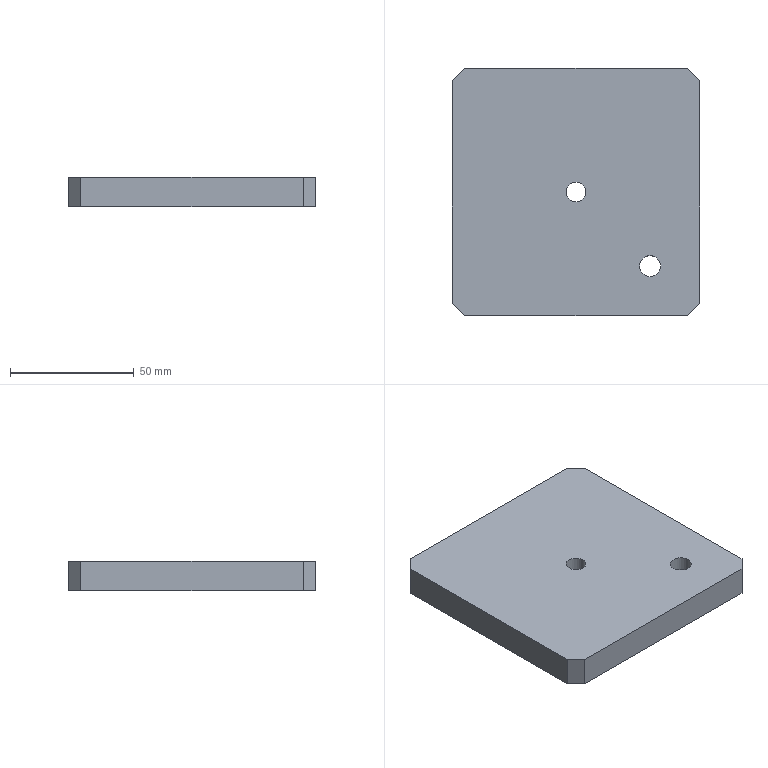Part | NX | features BREP 1 | 1 solid | 12 faces | box 100 x 100 x 12 mm | volume 118116 mm3 | plane 10 | cylinder 2 | commonest cylinder face diameters 8 x1 8.5 x1
STEP:
#1=CARTESIAN_POINT('',(50.,-45.,12.));
#2=VERTEX_POINT('',#1);
#3=CARTESIAN_POINT('',(50.,45.,12.));
#4=VERTEX_POINT('',#3);
#5=CARTESIAN_POINT('',(50.,-100.,12.));
#6=DIRECTION('',(0.,1.,0.));
#7=VECTOR('',#6,1000.);
#8=LINE('',#5,#7);
#9=EDGE_CURVE('',#2,#4,#8,.T.);
#10=ORIENTED_EDGE('',*,*,#9,.F.);
#11=CARTESIAN_POINT('',(50.,-45.,0.));
#12=VERTEX_POINT('',#11);
#13=CARTESIAN_POINT('',(50.,-45.,15.));
#14=DIRECTION('',(0.,0.,-1.));
#15=VECTOR('',#14,1000.);
#16=LINE('',#13,#15);
#17=EDGE_CURVE('',#2,#12,#16,.T.);
#18=ORIENTED_EDGE('',*,*,#17,.T.);
#19=CARTESIAN_POINT('',(50.,45.,0.));
#20=VERTEX_POINT('',#19);
#21=CARTESIAN_POINT('',(50.,50.,0.));
#22=DIRECTION('',(0.,1.,0.));
#23=VECTOR('',#22,1000.);
#24=LINE('',#21,#23);
#25=EDGE_CURVE('',#12,#20,#24,.T.);
#26=ORIENTED_EDGE('',*,*,#25,.T.);
#27=CARTESIAN_POINT('',(50.,45.,15.));
#28=DIRECTION('',(0.,0.,1.));
#29=VECTOR('',#28,1000.);
#30=LINE('',#27,#29);
#31=EDGE_CURVE('',#20,#4,#30,.T.);
#32=ORIENTED_EDGE('',*,*,#31,.T.);
#33=EDGE_LOOP('',(#10,#18,#26,#32));
#34=FACE_BOUND('',#33,.T.);
#35=CARTESIAN_POINT('',(50.,50.,15.));
#36=DIRECTION('',(-1.,0.,0.));
#37=DIRECTION('',(0.,0.,-1.));
#38=AXIS2_PLACEMENT_3D('',#35,#36,#37);
#39=PLANE('',#38);
#40=ADVANCED_FACE('',(#34),#39,.F.);
#41=CARTESIAN_POINT('',(45.,50.,12.));
#42=VERTEX_POINT('',#41);
#43=CARTESIAN_POINT('',(-45.,50.,12.));
#44=VERTEX_POINT('',#43);
#45=CARTESIAN_POINT('',(-50.,50.,12.));
#46=DIRECTION('',(-1.,0.,0.));
#47=VECTOR('',#46,1000.);
#48=LINE('',#45,#47);
#49=EDGE_CURVE('',#42,#44,#48,.T.);
#50=ORIENTED_EDGE('',*,*,#49,.F.);
#51=CARTESIAN_POINT('',(45.,50.,0.));
#52=VERTEX_POINT('',#51);
#53=CARTESIAN_POINT('',(45.,50.,15.));
#54=DIRECTION('',(0.,0.,-1.));
#55=VECTOR('',#54,1000.);
#56=LINE('',#53,#55);
#57=EDGE_CURVE('',#42,#52,#56,.T.);
#58=ORIENTED_EDGE('',*,*,#57,.T.);
#59=CARTESIAN_POINT('',(-45.,50.,0.));
#60=VERTEX_POINT('',#59);
#61=CARTESIAN_POINT('',(-50.,50.,0.));
#62=DIRECTION('',(-1.,0.,0.));
#63=VECTOR('',#62,1000.);
#64=LINE('',#61,#63);
#65=EDGE_CURVE('',#52,#60,#64,.T.);
#66=ORIENTED_EDGE('',*,*,#65,.T.);
#67=CARTESIAN_POINT('',(-45.,50.,15.));
#68=DIRECTION('',(0.,0.,1.));
#69=VECTOR('',#68,1000.);
#70=LINE('',#67,#69);
#71=EDGE_CURVE('',#60,#44,#70,.T.);
#72=ORIENTED_EDGE('',*,*,#71,.T.);
#73=EDGE_LOOP('',(#50,#58,#66,#72));
#74=FACE_BOUND('',#73,.T.);
#75=CARTESIAN_POINT('',(-50.,50.,15.));
#76=DIRECTION('',(0.,-1.,0.));
#77=DIRECTION('',(0.,0.,1.));
#78=AXIS2_PLACEMENT_3D('',#75,#76,#77);
#79=PLANE('',#78);
#80=ADVANCED_FACE('',(#74),#79,.F.);
#81=CARTESIAN_POINT('',(-50.,45.,12.));
#82=VERTEX_POINT('',#81);
#83=CARTESIAN_POINT('',(-50.,-45.,12.));
#84=VERTEX_POINT('',#83);
#85=CARTESIAN_POINT('',(-50.,50.,12.));
#86=DIRECTION('',(0.,-1.,0.));
#87=VECTOR('',#86,1000.);
#88=LINE('',#85,#87);
#89=EDGE_CURVE('',#82,#84,#88,.T.);
#90=ORIENTED_EDGE('',*,*,#89,.F.);
#91=CARTESIAN_POINT('',(-50.,45.,0.));
#92=VERTEX_POINT('',#91);
#93=CARTESIAN_POINT('',(-50.,45.,15.));
#94=DIRECTION('',(0.,0.,-1.));
#95=VECTOR('',#94,1000.);
#96=LINE('',#93,#95);
#97=EDGE_CURVE('',#82,#92,#96,.T.);
#98=ORIENTED_EDGE('',*,*,#97,.T.);
#99=CARTESIAN_POINT('',(-50.,-45.,0.));
#100=VERTEX_POINT('',#99);
#101=CARTESIAN_POINT('',(-50.,50.,0.));
#102=DIRECTION('',(0.,-1.,0.));
#103=VECTOR('',#102,1000.);
#104=LINE('',#101,#103);
#105=EDGE_CURVE('',#92,#100,#104,.T.);
#106=ORIENTED_EDGE('',*,*,#105,.T.);
#107=CARTESIAN_POINT('',(-50.,-45.,15.));
#108=DIRECTION('',(0.,0.,1.));
#109=VECTOR('',#108,1000.);
#110=LINE('',#107,#109);
#111=EDGE_CURVE('',#100,#84,#110,.T.);
#112=ORIENTED_EDGE('',*,*,#111,.T.);
#113=EDGE_LOOP('',(#90,#98,#106,#112));
#114=FACE_BOUND('',#113,.T.);
#115=CARTESIAN_POINT('',(-50.,50.,15.));
#116=DIRECTION('',(1.,0.,0.));
#117=DIRECTION('',(0.,-1.,0.));
#118=AXIS2_PLACEMENT_3D('',#115,#116,#117);
#119=PLANE('',#118);
#120=ADVANCED_FACE('',(#114),#119,.F.);
#121=CARTESIAN_POINT('',(-45.,-50.,12.));
#122=VERTEX_POINT('',#121);
#123=CARTESIAN_POINT('',(45.,-50.,12.));
#124=VERTEX_POINT('',#123);
#125=CARTESIAN_POINT('',(-50.,-50.,12.));
#126=DIRECTION('',(1.,0.,0.));
#127=VECTOR('',#126,1000.);
#128=LINE('',#125,#127);
#129=EDGE_CURVE('',#122,#124,#128,.T.);
#130=ORIENTED_EDGE('',*,*,#129,.F.);
#131=CARTESIAN_POINT('',(-45.,-50.,0.));
#132=VERTEX_POINT('',#131);
#133=CARTESIAN_POINT('',(-45.,-50.,15.));
#134=DIRECTION('',(0.,0.,-1.));
#135=VECTOR('',#134,1000.);
#136=LINE('',#133,#135);
#137=EDGE_CURVE('',#122,#132,#136,.T.);
#138=ORIENTED_EDGE('',*,*,#137,.T.);
#139=CARTESIAN_POINT('',(45.,-50.,0.));
#140=VERTEX_POINT('',#139);
#141=CARTESIAN_POINT('',(-50.,-50.,0.));
#142=DIRECTION('',(1.,0.,0.));
#143=VECTOR('',#142,1000.);
#144=LINE('',#141,#143);
#145=EDGE_CURVE('',#132,#140,#144,.T.);
#146=ORIENTED_EDGE('',*,*,#145,.T.);
#147=CARTESIAN_POINT('',(45.,-50.,15.));
#148=DIRECTION('',(0.,0.,1.));
#149=VECTOR('',#148,1000.);
#150=LINE('',#147,#149);
#151=EDGE_CURVE('',#140,#124,#150,.T.);
#152=ORIENTED_EDGE('',*,*,#151,.T.);
#153=EDGE_LOOP('',(#130,#138,#146,#152));
#154=FACE_BOUND('',#153,.T.);
#155=CARTESIAN_POINT('',(-50.,-50.,15.));
#156=DIRECTION('',(0.,1.,0.));
#157=DIRECTION('',(0.,0.,-1.));
#158=AXIS2_PLACEMENT_3D('',#155,#156,#157);
#159=PLANE('',#158);
#160=ADVANCED_FACE('',(#154),#159,.F.);
#161=ORIENTED_EDGE('',*,*,#137,.F.);
#162=CARTESIAN_POINT('',(-45.,-50.,12.));
#163=DIRECTION('',(-0.7071,0.7071,0.));
#164=VECTOR('',#163,1000.);
#165=LINE('',#162,#164);
#166=EDGE_CURVE('',#122,#84,#165,.T.);
#167=ORIENTED_EDGE('',*,*,#166,.T.);
#168=ORIENTED_EDGE('',*,*,#111,.F.);
#169=CARTESIAN_POINT('',(-45.,-50.,0.));
#170=DIRECTION('',(-0.7071,0.7071,0.));
#171=VECTOR('',#170,1000.);
#172=LINE('',#169,#171);
#173=EDGE_CURVE('',#132,#100,#172,.T.);
#174=ORIENTED_EDGE('',*,*,#173,.F.);
#175=EDGE_LOOP('',(#161,#167,#168,#174));
#176=FACE_BOUND('',#175,.T.);
#177=CARTESIAN_POINT('',(-45.,-50.,15.));
#178=DIRECTION('',(0.7071,0.7071,0.));
#179=DIRECTION('',(0.,0.,1.));
#180=AXIS2_PLACEMENT_3D('',#177,#178,#179);
#181=PLANE('',#180);
#182=ADVANCED_FACE('',(#176),#181,.F.);
#183=ORIENTED_EDGE('',*,*,#17,.F.);
#184=CARTESIAN_POINT('',(50.,-45.,12.));
#185=DIRECTION('',(-0.7071,-0.7071,0.));
#186=VECTOR('',#185,1000.);
#187=LINE('',#184,#186);
#188=EDGE_CURVE('',#2,#124,#187,.T.);
#189=ORIENTED_EDGE('',*,*,#188,.T.);
#190=ORIENTED_EDGE('',*,*,#151,.F.);
#191=CARTESIAN_POINT('',(50.,-45.,0.));
#192=DIRECTION('',(-0.7071,-0.7071,0.));
#193=VECTOR('',#192,1000.);
#194=LINE('',#191,#193);
#195=EDGE_CURVE('',#12,#140,#194,.T.);
#196=ORIENTED_EDGE('',*,*,#195,.F.);
#197=EDGE_LOOP('',(#183,#189,#190,#196));
#198=FACE_BOUND('',#197,.T.);
#199=CARTESIAN_POINT('',(50.,-45.,15.));
#200=DIRECTION('',(-0.7071,0.7071,0.));
#201=DIRECTION('',(0.,0.,1.));
#202=AXIS2_PLACEMENT_3D('',#199,#200,#201);
#203=PLANE('',#202);
#204=ADVANCED_FACE('',(#198),#203,.F.);
#205=ORIENTED_EDGE('',*,*,#57,.F.);
#206=CARTESIAN_POINT('',(45.,50.,12.));
#207=DIRECTION('',(0.7071,-0.7071,0.));
#208=VECTOR('',#207,1000.);
#209=LINE('',#206,#208);
#210=EDGE_CURVE('',#42,#4,#209,.T.);
#211=ORIENTED_EDGE('',*,*,#210,.T.);
#212=ORIENTED_EDGE('',*,*,#31,.F.);
#213=CARTESIAN_POINT('',(45.,50.,0.));
#214=DIRECTION('',(0.7071,-0.7071,0.));
#215=VECTOR('',#214,1000.);
#216=LINE('',#213,#215);
#217=EDGE_CURVE('',#52,#20,#216,.T.);
#218=ORIENTED_EDGE('',*,*,#217,.F.);
#219=EDGE_LOOP('',(#205,#211,#212,#218));
#220=FACE_BOUND('',#219,.T.);
#221=CARTESIAN_POINT('',(45.,50.,15.));
#222=DIRECTION('',(-0.7071,-0.7071,0.));
#223=DIRECTION('',(0.,0.,1.));
#224=AXIS2_PLACEMENT_3D('',#221,#222,#223);
#225=PLANE('',#224);
#226=ADVANCED_FACE('',(#220),#225,.F.);
#227=ORIENTED_EDGE('',*,*,#97,.F.);
#228=CARTESIAN_POINT('',(-50.,45.,12.));
#229=DIRECTION('',(0.7071,0.7071,0.));
#230=VECTOR('',#229,1000.);
#231=LINE('',#228,#230);
#232=EDGE_CURVE('',#82,#44,#231,.T.);
#233=ORIENTED_EDGE('',*,*,#232,.T.);
#234=ORIENTED_EDGE('',*,*,#71,.F.);
#235=CARTESIAN_POINT('',(-50.,45.,0.));
#236=DIRECTION('',(0.7071,0.7071,0.));
#237=VECTOR('',#236,1000.);
#238=LINE('',#235,#237);
#239=EDGE_CURVE('',#92,#60,#238,.T.);
#240=ORIENTED_EDGE('',*,*,#239,.F.);
#241=EDGE_LOOP('',(#227,#233,#234,#240));
#242=FACE_BOUND('',#241,.T.);
#243=CARTESIAN_POINT('',(-50.,45.,15.));
#244=DIRECTION('',(0.7071,-0.7071,0.));
#245=DIRECTION('',(0.,0.,1.));
#246=AXIS2_PLACEMENT_3D('',#243,#244,#245);
#247=PLANE('',#246);
#248=ADVANCED_FACE('',(#242),#247,.F.);
#249=CARTESIAN_POINT('',(34.25,-30.,0.));
#250=VERTEX_POINT('',#249);
#251=CARTESIAN_POINT('',(30.,-30.,0.));
#252=DIRECTION('',(0.,0.,1.));
#253=DIRECTION('',(1.,0.,0.));
#254=AXIS2_PLACEMENT_3D('',#251,#252,#253);
#255=CIRCLE('',#254,4.25);
#256=EDGE_CURVE('',#250,#250,#255,.T.);
#257=ORIENTED_EDGE('',*,*,#256,.T.);
#258=EDGE_LOOP('',(#257));
#259=FACE_BOUND('',#258,.T.);
#260=CARTESIAN_POINT('',(4.,0.,0.));
#261=VERTEX_POINT('',#260);
#262=CARTESIAN_POINT('',(0.,0.,0.));
#263=DIRECTION('',(0.,0.,1.));
#264=DIRECTION('',(1.,0.,0.));
#265=AXIS2_PLACEMENT_3D('',#262,#263,#264);
#266=CIRCLE('',#265,4.);
#267=EDGE_CURVE('',#261,#261,#266,.T.);
#268=ORIENTED_EDGE('',*,*,#267,.T.);
#269=EDGE_LOOP('',(#268));
#270=FACE_BOUND('',#269,.T.);
#271=ORIENTED_EDGE('',*,*,#145,.F.);
#272=ORIENTED_EDGE('',*,*,#173,.T.);
#273=ORIENTED_EDGE('',*,*,#105,.F.);
#274=ORIENTED_EDGE('',*,*,#239,.T.);
#275=ORIENTED_EDGE('',*,*,#65,.F.);
#276=ORIENTED_EDGE('',*,*,#217,.T.);
#277=ORIENTED_EDGE('',*,*,#25,.F.);
#278=ORIENTED_EDGE('',*,*,#195,.T.);
#279=EDGE_LOOP('',(#271,#272,#273,#274,#275,#276,#277,#278));
#280=FACE_BOUND('',#279,.T.);
#281=CARTESIAN_POINT('',(0.,0.,0.));
#282=DIRECTION('',(0.,0.,1.));
#283=DIRECTION('',(-1.,0.,0.));
#284=AXIS2_PLACEMENT_3D('',#281,#282,#283);
#285=PLANE('',#284);
#286=ADVANCED_FACE('',(#259,#270,#280),#285,.F.);
#287=CARTESIAN_POINT('',(34.25,-30.,12.));
#288=VERTEX_POINT('',#287);
#289=CARTESIAN_POINT('',(30.,-30.,12.));
#290=DIRECTION('',(0.,0.,1.));
#291=DIRECTION('',(1.,0.,0.));
#292=AXIS2_PLACEMENT_3D('',#289,#290,#291);
#293=CIRCLE('',#292,4.25);
#294=EDGE_CURVE('',#288,#288,#293,.T.);
#295=ORIENTED_EDGE('',*,*,#294,.F.);
#296=EDGE_LOOP('',(#295));
#297=FACE_BOUND('',#296,.T.);
#298=CARTESIAN_POINT('',(4.,0.,12.));
#299=VERTEX_POINT('',#298);
#300=CARTESIAN_POINT('',(0.,0.,12.));
#301=DIRECTION('',(0.,0.,1.));
#302=DIRECTION('',(1.,0.,0.));
#303=AXIS2_PLACEMENT_3D('',#300,#301,#302);
#304=CIRCLE('',#303,4.);
#305=EDGE_CURVE('',#299,#299,#304,.T.);
#306=ORIENTED_EDGE('',*,*,#305,.F.);
#307=EDGE_LOOP('',(#306));
#308=FACE_BOUND('',#307,.T.);
#309=ORIENTED_EDGE('',*,*,#9,.T.);
#310=ORIENTED_EDGE('',*,*,#210,.F.);
#311=ORIENTED_EDGE('',*,*,#49,.T.);
#312=ORIENTED_EDGE('',*,*,#232,.F.);
#313=ORIENTED_EDGE('',*,*,#89,.T.);
#314=ORIENTED_EDGE('',*,*,#166,.F.);
#315=ORIENTED_EDGE('',*,*,#129,.T.);
#316=ORIENTED_EDGE('',*,*,#188,.F.);
#317=EDGE_LOOP('',(#309,#310,#311,#312,#313,#314,#315,#316));
#318=FACE_BOUND('',#317,.T.);
#319=CARTESIAN_POINT('',(-900.,250.,12.));
#320=DIRECTION('',(0.,0.,1.));
#321=DIRECTION('',(-1.,0.,0.));
#322=AXIS2_PLACEMENT_3D('',#319,#320,#321);
#323=PLANE('',#322);
#324=ADVANCED_FACE('',(#297,#308,#318),#323,.T.);
#325=ORIENTED_EDGE('',*,*,#305,.T.);
#326=EDGE_LOOP('',(#325));
#327=FACE_BOUND('',#326,.T.);
#328=ORIENTED_EDGE('',*,*,#267,.F.);
#329=EDGE_LOOP('',(#328));
#330=FACE_BOUND('',#329,.T.);
#331=CARTESIAN_POINT('',(0.,0.,12.));
#332=DIRECTION('',(0.,0.,1.));
#333=DIRECTION('',(-1.,0.,0.));
#334=AXIS2_PLACEMENT_3D('',#331,#332,#333);
#335=CYLINDRICAL_SURFACE('',#334,4.);
#336=ADVANCED_FACE('',(#327,#330),#335,.F.);
#337=ORIENTED_EDGE('',*,*,#294,.T.);
#338=EDGE_LOOP('',(#337));
#339=FACE_BOUND('',#338,.T.);
#340=ORIENTED_EDGE('',*,*,#256,.F.);
#341=EDGE_LOOP('',(#340));
#342=FACE_BOUND('',#341,.T.);
#343=CARTESIAN_POINT('',(30.,-30.,12.));
#344=DIRECTION('',(0.,0.,1.));
#345=DIRECTION('',(-1.,0.,0.));
#346=AXIS2_PLACEMENT_3D('',#343,#344,#345);
#347=CYLINDRICAL_SURFACE('',#346,4.25);
#348=ADVANCED_FACE('',(#339,#342),#347,.F.);
#349=CLOSED_SHELL('',(#40,#80,#120,#160,#182,#204,#226,#248,#286,#324,#336,#348));
#350=MANIFOLD_SOLID_BREP('',#349);
#351=(LENGTH_UNIT()NAMED_UNIT(*)SI_UNIT(.MILLI.,.METRE.));
#352=UNCERTAINTY_MEASURE_WITH_UNIT(LENGTH_MEASURE(0.00001),#351,'','');
#353=(NAMED_UNIT(*)PLANE_ANGLE_UNIT()SI_UNIT($,.RADIAN.));
#354=(NAMED_UNIT(*)SI_UNIT($,.STERADIAN.)SOLID_ANGLE_UNIT());
#355=(GEOMETRIC_REPRESENTATION_CONTEXT(3)GLOBAL_UNCERTAINTY_ASSIGNED_CONTEXT((#352))GLOBAL_UNIT_ASSIGNED_CONTEXT((#351,#353,#354))REPRESENTATION_CONTEXT('',''));
#356=ADVANCED_BREP_SHAPE_REPRESENTATION('',(#350),#355);